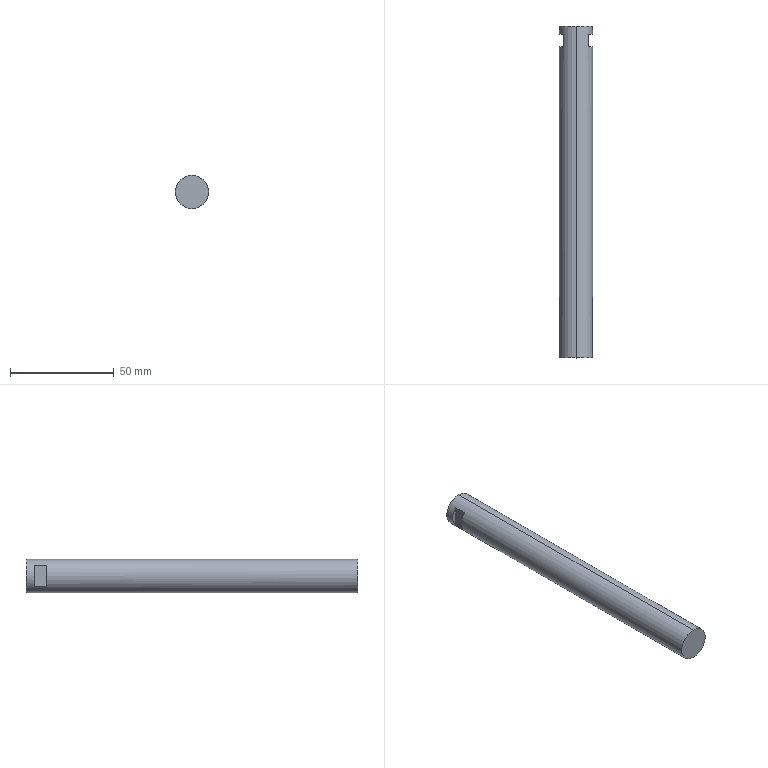Part | STEP file | 1 solid | 10 faces | box 16 x 160 x 16 mm | volume 31996 mm3 | plane 8 | cylinder 2 | commonest cylinder face diameters 16 x2
STEP:
#1=CARTESIAN_POINT('',(0.,0.,0.));
#2=DIRECTION('',(0.,0.,1.));
#3=DIRECTION('',(1.,0.,0.));
#4=AXIS2_PLACEMENT_3D('',#1,#2,#3);
#5=CARTESIAN_POINT('',(6.,156.,5.292));
#6=VERTEX_POINT('',#5);
#7=CARTESIAN_POINT('',(6.,156.,-5.292));
#8=VERTEX_POINT('',#7);
#9=CARTESIAN_POINT('',(0.,156.,0.));
#10=DIRECTION('',(0.,1.,0.));
#11=DIRECTION('',(0.,0.,1.));
#12=AXIS2_PLACEMENT_3D('',#9,#10,#11);
#13=CIRCLE('',#12,8.);
#14=CARTESIAN_POINT('',(0.,160.,0.));
#15=DIRECTION('',(0.,-1.,0.));
#16=DIRECTION('',(0.,0.,-1.));
#17=AXIS2_PLACEMENT_3D('',#14,#15,#16);
#18=CYLINDRICAL_SURFACE('',#17,8.);
#19=CARTESIAN_POINT('',(3.142,4.));
#20=DIRECTION('',(-1.,0.));
#21=VECTOR('',#20,1.);
#22=LINE('',#19,#21);
#23=(GEOMETRIC_REPRESENTATION_CONTEXT(2)PARAMETRIC_REPRESENTATION_CONTEXT()REPRESENTATION_CONTEXT('',''));
#24=DEFINITIONAL_REPRESENTATION('',(#22),#23);
#25=PCURVE('',#18,#24);
#26=CARTESIAN_POINT('',(14.,156.,-12.));
#27=DIRECTION('',(0.,1.,0.));
#28=DIRECTION('',(0.,0.,1.));
#29=AXIS2_PLACEMENT_3D('',#26,#27,#28);
#30=PLANE('',#29);
#31=CARTESIAN_POINT('',(12.,-14.));
#32=DIRECTION('',(1.,0.));
#33=AXIS2_PLACEMENT_2D('',#31,#32);
#34=CIRCLE('',#33,8.);
#35=(GEOMETRIC_REPRESENTATION_CONTEXT(2)PARAMETRIC_REPRESENTATION_CONTEXT()REPRESENTATION_CONTEXT('',''));
#36=DEFINITIONAL_REPRESENTATION('',(#34),#35);
#37=PCURVE('',#30,#36);
#38=SURFACE_CURVE('',#13,(#25,#37),.PCURVE_S1.);
#39=EDGE_CURVE('',#6,#8,#38,.T.);
#40=ORIENTED_EDGE('',*,*,#39,.T.);
#41=CARTESIAN_POINT('',(6.,150.,-5.292));
#42=VERTEX_POINT('',#41);
#43=CARTESIAN_POINT('',(6.,160.,-5.292));
#44=DIRECTION('',(0.,-1.,0.));
#45=VECTOR('',#44,1.);
#46=LINE('',#43,#45);
#47=CARTESIAN_POINT('',(0.8481,0.));
#48=DIRECTION('',(0.,1.));
#49=VECTOR('',#48,1.);
#50=LINE('',#47,#49);
#51=(GEOMETRIC_REPRESENTATION_CONTEXT(2)PARAMETRIC_REPRESENTATION_CONTEXT()REPRESENTATION_CONTEXT('',''));
#52=DEFINITIONAL_REPRESENTATION('',(#50),#51);
#53=PCURVE('',#18,#52);
#54=CARTESIAN_POINT('',(6.,156.,-12.));
#55=DIRECTION('',(-1.,0.,0.));
#56=DIRECTION('',(0.,-1.,0.));
#57=AXIS2_PLACEMENT_3D('',#54,#55,#56);
#58=PLANE('',#57);
#59=CARTESIAN_POINT('',(-4.,6.708));
#60=DIRECTION('',(1.,0.));
#61=VECTOR('',#60,1.);
#62=LINE('',#59,#61);
#63=(GEOMETRIC_REPRESENTATION_CONTEXT(2)PARAMETRIC_REPRESENTATION_CONTEXT()REPRESENTATION_CONTEXT('',''));
#64=DEFINITIONAL_REPRESENTATION('',(#62),#63);
#65=PCURVE('',#58,#64);
#66=SURFACE_CURVE('',#46,(#53,#65),.PCURVE_S1.);
#67=EDGE_CURVE('',#8,#42,#66,.T.);
#68=ORIENTED_EDGE('',*,*,#67,.T.);
#69=CARTESIAN_POINT('',(6.,150.,5.292));
#70=VERTEX_POINT('',#69);
#71=CARTESIAN_POINT('',(0.,150.,0.));
#72=DIRECTION('',(0.,-1.,0.));
#73=DIRECTION('',(0.,0.,-1.));
#74=AXIS2_PLACEMENT_3D('',#71,#72,#73);
#75=CIRCLE('',#74,8.);
#76=CARTESIAN_POINT('',(0.,10.));
#77=DIRECTION('',(1.,0.));
#78=VECTOR('',#77,1.);
#79=LINE('',#76,#78);
#80=(GEOMETRIC_REPRESENTATION_CONTEXT(2)PARAMETRIC_REPRESENTATION_CONTEXT()REPRESENTATION_CONTEXT('',''));
#81=DEFINITIONAL_REPRESENTATION('',(#79),#80);
#82=PCURVE('',#18,#81);
#83=CARTESIAN_POINT('',(14.,150.,-12.));
#84=DIRECTION('',(0.,-1.,0.));
#85=DIRECTION('',(0.,0.,-1.));
#86=AXIS2_PLACEMENT_3D('',#83,#84,#85);
#87=PLANE('',#86);
#88=CARTESIAN_POINT('',(-12.,-14.));
#89=DIRECTION('',(1.,0.));
#90=AXIS2_PLACEMENT_2D('',#88,#89);
#91=CIRCLE('',#90,8.);
#92=(GEOMETRIC_REPRESENTATION_CONTEXT(2)PARAMETRIC_REPRESENTATION_CONTEXT()REPRESENTATION_CONTEXT('',''));
#93=DEFINITIONAL_REPRESENTATION('',(#91),#92);
#94=PCURVE('',#87,#93);
#95=SURFACE_CURVE('',#75,(#82,#94),.PCURVE_S1.);
#96=EDGE_CURVE('',#42,#70,#95,.T.);
#97=ORIENTED_EDGE('',*,*,#96,.T.);
#98=CARTESIAN_POINT('',(6.,160.,5.292));
#99=DIRECTION('',(0.,1.,0.));
#100=VECTOR('',#99,1.);
#101=LINE('',#98,#100);
#102=CARTESIAN_POINT('',(2.294,0.));
#103=DIRECTION('',(0.,-1.));
#104=VECTOR('',#103,1.);
#105=LINE('',#102,#104);
#106=(GEOMETRIC_REPRESENTATION_CONTEXT(2)PARAMETRIC_REPRESENTATION_CONTEXT()REPRESENTATION_CONTEXT('',''));
#107=DEFINITIONAL_REPRESENTATION('',(#105),#106);
#108=PCURVE('',#18,#107);
#109=CARTESIAN_POINT('',(-4.,17.292));
#110=DIRECTION('',(-1.,0.));
#111=VECTOR('',#110,1.);
#112=LINE('',#109,#111);
#113=(GEOMETRIC_REPRESENTATION_CONTEXT(2)PARAMETRIC_REPRESENTATION_CONTEXT()REPRESENTATION_CONTEXT('',''));
#114=DEFINITIONAL_REPRESENTATION('',(#112),#113);
#115=PCURVE('',#58,#114);
#116=SURFACE_CURVE('',#101,(#108,#115),.PCURVE_S1.);
#117=EDGE_CURVE('',#70,#6,#116,.T.);
#118=ORIENTED_EDGE('',*,*,#117,.T.);
#119=EDGE_LOOP('',(#40,#68,#97,#118));
#120=FACE_BOUND('',#119,.T.);
#121=CARTESIAN_POINT('',(0.,160.,8.));
#122=VERTEX_POINT('',#121);
#123=CARTESIAN_POINT('',(0.,160.,-8.));
#124=VERTEX_POINT('',#123);
#125=CARTESIAN_POINT('',(0.,160.,0.));
#126=DIRECTION('',(0.,1.,0.));
#127=DIRECTION('',(0.,0.,1.));
#128=AXIS2_PLACEMENT_3D('',#125,#126,#127);
#129=CIRCLE('',#128,8.);
#130=CARTESIAN_POINT('',(3.142,0.));
#131=DIRECTION('',(-1.,0.));
#132=VECTOR('',#131,1.);
#133=LINE('',#130,#132);
#134=(GEOMETRIC_REPRESENTATION_CONTEXT(2)PARAMETRIC_REPRESENTATION_CONTEXT()REPRESENTATION_CONTEXT('',''));
#135=DEFINITIONAL_REPRESENTATION('',(#133),#134);
#136=PCURVE('',#18,#135);
#137=CARTESIAN_POINT('',(0.,160.,0.));
#138=DIRECTION('',(0.,1.,0.));
#139=DIRECTION('',(0.,0.,1.));
#140=AXIS2_PLACEMENT_3D('',#137,#138,#139);
#141=PLANE('',#140);
#142=CARTESIAN_POINT('',(0.,0.));
#143=DIRECTION('',(1.,0.));
#144=AXIS2_PLACEMENT_2D('',#142,#143);
#145=CIRCLE('',#144,8.);
#146=(GEOMETRIC_REPRESENTATION_CONTEXT(2)PARAMETRIC_REPRESENTATION_CONTEXT()REPRESENTATION_CONTEXT('',''));
#147=DEFINITIONAL_REPRESENTATION('',(#145),#146);
#148=PCURVE('',#141,#147);
#149=SURFACE_CURVE('',#129,(#136,#148),.PCURVE_S1.);
#150=EDGE_CURVE('',#122,#124,#149,.T.);
#151=ORIENTED_EDGE('',*,*,#150,.F.);
#152=CARTESIAN_POINT('',(0.,0.,8.));
#153=VERTEX_POINT('',#152);
#154=CARTESIAN_POINT('',(0.,160.,8.));
#155=DIRECTION('',(0.,-1.,0.));
#156=VECTOR('',#155,1.);
#157=LINE('',#154,#156);
#158=CARTESIAN_POINT('',(3.142,0.));
#159=DIRECTION('',(0.,1.));
#160=VECTOR('',#159,1.);
#161=LINE('',#158,#160);
#162=(GEOMETRIC_REPRESENTATION_CONTEXT(2)PARAMETRIC_REPRESENTATION_CONTEXT()REPRESENTATION_CONTEXT('',''));
#163=DEFINITIONAL_REPRESENTATION('',(#161),#162);
#164=PCURVE('',#18,#163);
#165=CARTESIAN_POINT('',(0.,160.,0.));
#166=DIRECTION('',(0.,-1.,0.));
#167=DIRECTION('',(0.,0.,-1.));
#168=AXIS2_PLACEMENT_3D('',#165,#166,#167);
#169=CYLINDRICAL_SURFACE('',#168,8.);
#170=CARTESIAN_POINT('',(3.142,0.));
#171=DIRECTION('',(0.,1.));
#172=VECTOR('',#171,1.);
#173=LINE('',#170,#172);
#174=(GEOMETRIC_REPRESENTATION_CONTEXT(2)PARAMETRIC_REPRESENTATION_CONTEXT()REPRESENTATION_CONTEXT('',''));
#175=DEFINITIONAL_REPRESENTATION('',(#173),#174);
#176=PCURVE('',#169,#175);
#177=SURFACE_CURVE('',#157,(#164,#176),.PCURVE_S1.);
#178=EDGE_CURVE('',#122,#153,#177,.T.);
#179=ORIENTED_EDGE('',*,*,#178,.T.);
#180=CARTESIAN_POINT('',(0.,0.,-8.));
#181=VERTEX_POINT('',#180);
#182=CARTESIAN_POINT('',(0.,0.,0.));
#183=DIRECTION('',(0.,1.,0.));
#184=DIRECTION('',(0.,0.,1.));
#185=AXIS2_PLACEMENT_3D('',#182,#183,#184);
#186=CIRCLE('',#185,8.);
#187=CARTESIAN_POINT('',(3.142,160.));
#188=DIRECTION('',(-1.,0.));
#189=VECTOR('',#188,1.);
#190=LINE('',#187,#189);
#191=(GEOMETRIC_REPRESENTATION_CONTEXT(2)PARAMETRIC_REPRESENTATION_CONTEXT()REPRESENTATION_CONTEXT('',''));
#192=DEFINITIONAL_REPRESENTATION('',(#190),#191);
#193=PCURVE('',#18,#192);
#194=CARTESIAN_POINT('',(0.,0.,0.));
#195=DIRECTION('',(0.,1.,0.));
#196=DIRECTION('',(0.,0.,1.));
#197=AXIS2_PLACEMENT_3D('',#194,#195,#196);
#198=PLANE('',#197);
#199=CARTESIAN_POINT('',(0.,0.));
#200=DIRECTION('',(1.,0.));
#201=AXIS2_PLACEMENT_2D('',#199,#200);
#202=CIRCLE('',#201,8.);
#203=(GEOMETRIC_REPRESENTATION_CONTEXT(2)PARAMETRIC_REPRESENTATION_CONTEXT()REPRESENTATION_CONTEXT('',''));
#204=DEFINITIONAL_REPRESENTATION('',(#202),#203);
#205=PCURVE('',#198,#204);
#206=SURFACE_CURVE('',#186,(#193,#205),.PCURVE_S1.);
#207=EDGE_CURVE('',#153,#181,#206,.T.);
#208=ORIENTED_EDGE('',*,*,#207,.T.);
#209=CARTESIAN_POINT('',(0.,160.,-8.));
#210=DIRECTION('',(0.,-1.,0.));
#211=VECTOR('',#210,1.);
#212=LINE('',#209,#211);
#213=CARTESIAN_POINT('',(0.,0.));
#214=DIRECTION('',(0.,1.));
#215=VECTOR('',#214,1.);
#216=LINE('',#213,#215);
#217=(GEOMETRIC_REPRESENTATION_CONTEXT(2)PARAMETRIC_REPRESENTATION_CONTEXT()REPRESENTATION_CONTEXT('',''));
#218=DEFINITIONAL_REPRESENTATION('',(#216),#217);
#219=PCURVE('',#18,#218);
#220=CARTESIAN_POINT('',(6.283,0.));
#221=DIRECTION('',(0.,1.));
#222=VECTOR('',#221,1.);
#223=LINE('',#220,#222);
#224=(GEOMETRIC_REPRESENTATION_CONTEXT(2)PARAMETRIC_REPRESENTATION_CONTEXT()REPRESENTATION_CONTEXT('',''));
#225=DEFINITIONAL_REPRESENTATION('',(#223),#224);
#226=PCURVE('',#169,#225);
#227=SURFACE_CURVE('',#212,(#219,#226),.PCURVE_S1.);
#228=EDGE_CURVE('',#124,#181,#227,.T.);
#229=ORIENTED_EDGE('',*,*,#228,.F.);
#230=EDGE_LOOP('',(#151,#179,#208,#229));
#231=FACE_BOUND('',#230,.T.);
#232=ADVANCED_FACE('',(#120,#231),#18,.T.);
#233=ORIENTED_EDGE('',*,*,#178,.F.);
#234=CARTESIAN_POINT('',(0.,160.,0.));
#235=DIRECTION('',(0.,1.,0.));
#236=DIRECTION('',(0.,0.,1.));
#237=AXIS2_PLACEMENT_3D('',#234,#235,#236);
#238=CIRCLE('',#237,8.);
#239=CARTESIAN_POINT('',(9.425,0.));
#240=DIRECTION('',(-1.,0.));
#241=VECTOR('',#240,1.);
#242=LINE('',#239,#241);
#243=(GEOMETRIC_REPRESENTATION_CONTEXT(2)PARAMETRIC_REPRESENTATION_CONTEXT()REPRESENTATION_CONTEXT('',''));
#244=DEFINITIONAL_REPRESENTATION('',(#242),#243);
#245=PCURVE('',#169,#244);
#246=CARTESIAN_POINT('',(0.,0.));
#247=DIRECTION('',(1.,0.));
#248=AXIS2_PLACEMENT_2D('',#246,#247);
#249=CIRCLE('',#248,8.);
#250=(GEOMETRIC_REPRESENTATION_CONTEXT(2)PARAMETRIC_REPRESENTATION_CONTEXT()REPRESENTATION_CONTEXT('',''));
#251=DEFINITIONAL_REPRESENTATION('',(#249),#250);
#252=PCURVE('',#141,#251);
#253=SURFACE_CURVE('',#238,(#245,#252),.PCURVE_S1.);
#254=EDGE_CURVE('',#124,#122,#253,.T.);
#255=ORIENTED_EDGE('',*,*,#254,.F.);
#256=ORIENTED_EDGE('',*,*,#228,.T.);
#257=CARTESIAN_POINT('',(0.,0.,0.));
#258=DIRECTION('',(0.,1.,0.));
#259=DIRECTION('',(0.,0.,1.));
#260=AXIS2_PLACEMENT_3D('',#257,#258,#259);
#261=CIRCLE('',#260,8.);
#262=CARTESIAN_POINT('',(9.425,160.));
#263=DIRECTION('',(-1.,0.));
#264=VECTOR('',#263,1.);
#265=LINE('',#262,#264);
#266=(GEOMETRIC_REPRESENTATION_CONTEXT(2)PARAMETRIC_REPRESENTATION_CONTEXT()REPRESENTATION_CONTEXT('',''));
#267=DEFINITIONAL_REPRESENTATION('',(#265),#266);
#268=PCURVE('',#169,#267);
#269=CARTESIAN_POINT('',(0.,0.));
#270=DIRECTION('',(1.,0.));
#271=AXIS2_PLACEMENT_2D('',#269,#270);
#272=CIRCLE('',#271,8.);
#273=(GEOMETRIC_REPRESENTATION_CONTEXT(2)PARAMETRIC_REPRESENTATION_CONTEXT()REPRESENTATION_CONTEXT('',''));
#274=DEFINITIONAL_REPRESENTATION('',(#272),#273);
#275=PCURVE('',#198,#274);
#276=SURFACE_CURVE('',#261,(#268,#275),.PCURVE_S1.);
#277=EDGE_CURVE('',#181,#153,#276,.T.);
#278=ORIENTED_EDGE('',*,*,#277,.T.);
#279=EDGE_LOOP('',(#233,#255,#256,#278));
#280=FACE_BOUND('',#279,.T.);
#281=CARTESIAN_POINT('',(-6.,150.,-5.292));
#282=VERTEX_POINT('',#281);
#283=CARTESIAN_POINT('',(-6.,156.,-5.292));
#284=VERTEX_POINT('',#283);
#285=CARTESIAN_POINT('',(-6.,160.,-5.292));
#286=DIRECTION('',(0.,1.,0.));
#287=VECTOR('',#286,1.);
#288=LINE('',#285,#287);
#289=CARTESIAN_POINT('',(5.435,0.));
#290=DIRECTION('',(0.,-1.));
#291=VECTOR('',#290,1.);
#292=LINE('',#289,#291);
#293=(GEOMETRIC_REPRESENTATION_CONTEXT(2)PARAMETRIC_REPRESENTATION_CONTEXT()REPRESENTATION_CONTEXT('',''));
#294=DEFINITIONAL_REPRESENTATION('',(#292),#293);
#295=PCURVE('',#169,#294);
#296=CARTESIAN_POINT('',(-6.,156.,-12.));
#297=DIRECTION('',(1.,0.,0.));
#298=DIRECTION('',(0.,1.,0.));
#299=AXIS2_PLACEMENT_3D('',#296,#297,#298);
#300=PLANE('',#299);
#301=CARTESIAN_POINT('',(4.,6.708));
#302=DIRECTION('',(1.,0.));
#303=VECTOR('',#302,1.);
#304=LINE('',#301,#303);
#305=(GEOMETRIC_REPRESENTATION_CONTEXT(2)PARAMETRIC_REPRESENTATION_CONTEXT()REPRESENTATION_CONTEXT('',''));
#306=DEFINITIONAL_REPRESENTATION('',(#304),#305);
#307=PCURVE('',#300,#306);
#308=SURFACE_CURVE('',#288,(#295,#307),.PCURVE_S1.);
#309=EDGE_CURVE('',#282,#284,#308,.T.);
#310=ORIENTED_EDGE('',*,*,#309,.T.);
#311=CARTESIAN_POINT('',(-6.,156.,5.292));
#312=VERTEX_POINT('',#311);
#313=CARTESIAN_POINT('',(0.,156.,0.));
#314=DIRECTION('',(0.,1.,0.));
#315=DIRECTION('',(0.,0.,1.));
#316=AXIS2_PLACEMENT_3D('',#313,#314,#315);
#317=CIRCLE('',#316,8.);
#318=CARTESIAN_POINT('',(9.425,4.));
#319=DIRECTION('',(-1.,0.));
#320=VECTOR('',#319,1.);
#321=LINE('',#318,#320);
#322=(GEOMETRIC_REPRESENTATION_CONTEXT(2)PARAMETRIC_REPRESENTATION_CONTEXT()REPRESENTATION_CONTEXT('',''));
#323=DEFINITIONAL_REPRESENTATION('',(#321),#322);
#324=PCURVE('',#169,#323);
#325=CARTESIAN_POINT('',(-14.,156.,-12.));
#326=DIRECTION('',(0.,1.,0.));
#327=DIRECTION('',(0.,0.,1.));
#328=AXIS2_PLACEMENT_3D('',#325,#326,#327);
#329=PLANE('',#328);
#330=CARTESIAN_POINT('',(12.,14.));
#331=DIRECTION('',(1.,0.));
#332=AXIS2_PLACEMENT_2D('',#330,#331);
#333=CIRCLE('',#332,8.);
#334=(GEOMETRIC_REPRESENTATION_CONTEXT(2)PARAMETRIC_REPRESENTATION_CONTEXT()REPRESENTATION_CONTEXT('',''));
#335=DEFINITIONAL_REPRESENTATION('',(#333),#334);
#336=PCURVE('',#329,#335);
#337=SURFACE_CURVE('',#317,(#324,#336),.PCURVE_S1.);
#338=EDGE_CURVE('',#284,#312,#337,.T.);
#339=ORIENTED_EDGE('',*,*,#338,.T.);
#340=CARTESIAN_POINT('',(-6.,150.,5.292));
#341=VERTEX_POINT('',#340);
#342=CARTESIAN_POINT('',(-6.,160.,5.292));
#343=DIRECTION('',(0.,-1.,0.));
#344=VECTOR('',#343,1.);
#345=LINE('',#342,#344);
#346=CARTESIAN_POINT('',(3.99,0.));
#347=DIRECTION('',(0.,1.));
#348=VECTOR('',#347,1.);
#349=LINE('',#346,#348);
#350=(GEOMETRIC_REPRESENTATION_CONTEXT(2)PARAMETRIC_REPRESENTATION_CONTEXT()REPRESENTATION_CONTEXT('',''));
#351=DEFINITIONAL_REPRESENTATION('',(#349),#350);
#352=PCURVE('',#169,#351);
#353=CARTESIAN_POINT('',(4.,17.292));
#354=DIRECTION('',(-1.,0.));
#355=VECTOR('',#354,1.);
#356=LINE('',#353,#355);
#357=(GEOMETRIC_REPRESENTATION_CONTEXT(2)PARAMETRIC_REPRESENTATION_CONTEXT()REPRESENTATION_CONTEXT('',''));
#358=DEFINITIONAL_REPRESENTATION('',(#356),#357);
#359=PCURVE('',#300,#358);
#360=SURFACE_CURVE('',#345,(#352,#359),.PCURVE_S1.);
#361=EDGE_CURVE('',#312,#341,#360,.T.);
#362=ORIENTED_EDGE('',*,*,#361,.T.);
#363=CARTESIAN_POINT('',(0.,150.,0.));
#364=DIRECTION('',(0.,-1.,0.));
#365=DIRECTION('',(0.,0.,-1.));
#366=AXIS2_PLACEMENT_3D('',#363,#364,#365);
#367=CIRCLE('',#366,8.);
#368=CARTESIAN_POINT('',(0.,10.));
#369=DIRECTION('',(1.,0.));
#370=VECTOR('',#369,1.);
#371=LINE('',#368,#370);
#372=(GEOMETRIC_REPRESENTATION_CONTEXT(2)PARAMETRIC_REPRESENTATION_CONTEXT()REPRESENTATION_CONTEXT('',''));
#373=DEFINITIONAL_REPRESENTATION('',(#371),#372);
#374=PCURVE('',#169,#373);
#375=CARTESIAN_POINT('',(-14.,150.,-12.));
#376=DIRECTION('',(0.,-1.,0.));
#377=DIRECTION('',(0.,0.,-1.));
#378=AXIS2_PLACEMENT_3D('',#375,#376,#377);
#379=PLANE('',#378);
#380=CARTESIAN_POINT('',(-12.,14.));
#381=DIRECTION('',(1.,0.));
#382=AXIS2_PLACEMENT_2D('',#380,#381);
#383=CIRCLE('',#382,8.);
#384=(GEOMETRIC_REPRESENTATION_CONTEXT(2)PARAMETRIC_REPRESENTATION_CONTEXT()REPRESENTATION_CONTEXT('',''));
#385=DEFINITIONAL_REPRESENTATION('',(#383),#384);
#386=PCURVE('',#379,#385);
#387=SURFACE_CURVE('',#367,(#374,#386),.PCURVE_S1.);
#388=EDGE_CURVE('',#341,#282,#387,.T.);
#389=ORIENTED_EDGE('',*,*,#388,.T.);
#390=EDGE_LOOP('',(#310,#339,#362,#389));
#391=FACE_BOUND('',#390,.T.);
#392=ADVANCED_FACE('',(#280,#391),#169,.T.);
#393=ORIENTED_EDGE('',*,*,#254,.T.);
#394=ORIENTED_EDGE('',*,*,#150,.T.);
#395=EDGE_LOOP('',(#393,#394));
#396=FACE_BOUND('',#395,.T.);
#397=ADVANCED_FACE('',(#396),#141,.T.);
#398=ORIENTED_EDGE('',*,*,#277,.F.);
#399=ORIENTED_EDGE('',*,*,#207,.F.);
#400=EDGE_LOOP('',(#398,#399));
#401=FACE_BOUND('',#400,.T.);
#402=ADVANCED_FACE('',(#401),#198,.F.);
#403=CARTESIAN_POINT('',(-6.,156.,-12.));
#404=DIRECTION('',(0.,0.,1.));
#405=VECTOR('',#404,1.);
#406=LINE('',#403,#405);
#407=CARTESIAN_POINT('',(0.,8.));
#408=DIRECTION('',(1.,0.));
#409=VECTOR('',#408,1.);
#410=LINE('',#407,#409);
#411=(GEOMETRIC_REPRESENTATION_CONTEXT(2)PARAMETRIC_REPRESENTATION_CONTEXT()REPRESENTATION_CONTEXT('',''));
#412=DEFINITIONAL_REPRESENTATION('',(#410),#411);
#413=PCURVE('',#329,#412);
#414=CARTESIAN_POINT('',(0.,0.));
#415=DIRECTION('',(0.,1.));
#416=VECTOR('',#415,1.);
#417=LINE('',#414,#416);
#418=(GEOMETRIC_REPRESENTATION_CONTEXT(2)PARAMETRIC_REPRESENTATION_CONTEXT()REPRESENTATION_CONTEXT('',''));
#419=DEFINITIONAL_REPRESENTATION('',(#417),#418);
#420=PCURVE('',#300,#419);
#421=SURFACE_CURVE('',#406,(#413,#420),.PCURVE_S1.);
#422=EDGE_CURVE('',#284,#312,#421,.T.);
#423=ORIENTED_EDGE('',*,*,#422,.T.);
#424=ORIENTED_EDGE('',*,*,#338,.F.);
#425=EDGE_LOOP('',(#423,#424));
#426=FACE_BOUND('',#425,.T.);
#427=ADVANCED_FACE('',(#426),#329,.F.);
#428=ORIENTED_EDGE('',*,*,#422,.F.);
#429=ORIENTED_EDGE('',*,*,#309,.F.);
#430=CARTESIAN_POINT('',(-6.,150.,-12.));
#431=DIRECTION('',(0.,0.,1.));
#432=VECTOR('',#431,1.);
#433=LINE('',#430,#432);
#434=CARTESIAN_POINT('',(-6.,0.));
#435=DIRECTION('',(0.,1.));
#436=VECTOR('',#435,1.);
#437=LINE('',#434,#436);
#438=(GEOMETRIC_REPRESENTATION_CONTEXT(2)PARAMETRIC_REPRESENTATION_CONTEXT()REPRESENTATION_CONTEXT('',''));
#439=DEFINITIONAL_REPRESENTATION('',(#437),#438);
#440=PCURVE('',#300,#439);
#441=CARTESIAN_POINT('',(0.,8.));
#442=DIRECTION('',(-1.,0.));
#443=VECTOR('',#442,1.);
#444=LINE('',#441,#443);
#445=(GEOMETRIC_REPRESENTATION_CONTEXT(2)PARAMETRIC_REPRESENTATION_CONTEXT()REPRESENTATION_CONTEXT('',''));
#446=DEFINITIONAL_REPRESENTATION('',(#444),#445);
#447=PCURVE('',#379,#446);
#448=SURFACE_CURVE('',#433,(#440,#447),.PCURVE_S1.);
#449=EDGE_CURVE('',#282,#341,#448,.T.);
#450=ORIENTED_EDGE('',*,*,#449,.T.);
#451=ORIENTED_EDGE('',*,*,#361,.F.);
#452=EDGE_LOOP('',(#428,#429,#450,#451));
#453=FACE_BOUND('',#452,.T.);
#454=ADVANCED_FACE('',(#453),#300,.F.);
#455=ORIENTED_EDGE('',*,*,#449,.F.);
#456=ORIENTED_EDGE('',*,*,#388,.F.);
#457=EDGE_LOOP('',(#455,#456));
#458=FACE_BOUND('',#457,.T.);
#459=ADVANCED_FACE('',(#458),#379,.F.);
#460=CARTESIAN_POINT('',(6.,156.,-12.));
#461=DIRECTION('',(0.,0.,1.));
#462=VECTOR('',#461,1.);
#463=LINE('',#460,#462);
#464=CARTESIAN_POINT('',(0.,-8.));
#465=DIRECTION('',(1.,0.));
#466=VECTOR('',#465,1.);
#467=LINE('',#464,#466);
#468=(GEOMETRIC_REPRESENTATION_CONTEXT(2)PARAMETRIC_REPRESENTATION_CONTEXT()REPRESENTATION_CONTEXT('',''));
#469=DEFINITIONAL_REPRESENTATION('',(#467),#468);
#470=PCURVE('',#30,#469);
#471=CARTESIAN_POINT('',(0.,0.));
#472=DIRECTION('',(0.,1.));
#473=VECTOR('',#472,1.);
#474=LINE('',#471,#473);
#475=(GEOMETRIC_REPRESENTATION_CONTEXT(2)PARAMETRIC_REPRESENTATION_CONTEXT()REPRESENTATION_CONTEXT('',''));
#476=DEFINITIONAL_REPRESENTATION('',(#474),#475);
#477=PCURVE('',#58,#476);
#478=SURFACE_CURVE('',#463,(#470,#477),.PCURVE_S1.);
#479=EDGE_CURVE('',#8,#6,#478,.T.);
#480=ORIENTED_EDGE('',*,*,#479,.F.);
#481=ORIENTED_EDGE('',*,*,#39,.F.);
#482=EDGE_LOOP('',(#480,#481));
#483=FACE_BOUND('',#482,.T.);
#484=ADVANCED_FACE('',(#483),#30,.F.);
#485=CARTESIAN_POINT('',(6.,150.,-12.));
#486=DIRECTION('',(0.,0.,1.));
#487=VECTOR('',#486,1.);
#488=LINE('',#485,#487);
#489=CARTESIAN_POINT('',(0.,-8.));
#490=DIRECTION('',(-1.,0.));
#491=VECTOR('',#490,1.);
#492=LINE('',#489,#491);
#493=(GEOMETRIC_REPRESENTATION_CONTEXT(2)PARAMETRIC_REPRESENTATION_CONTEXT()REPRESENTATION_CONTEXT('',''));
#494=DEFINITIONAL_REPRESENTATION('',(#492),#493);
#495=PCURVE('',#87,#494);
#496=CARTESIAN_POINT('',(6.,0.));
#497=DIRECTION('',(0.,1.));
#498=VECTOR('',#497,1.);
#499=LINE('',#496,#498);
#500=(GEOMETRIC_REPRESENTATION_CONTEXT(2)PARAMETRIC_REPRESENTATION_CONTEXT()REPRESENTATION_CONTEXT('',''));
#501=DEFINITIONAL_REPRESENTATION('',(#499),#500);
#502=PCURVE('',#58,#501);
#503=SURFACE_CURVE('',#488,(#495,#502),.PCURVE_S1.);
#504=EDGE_CURVE('',#42,#70,#503,.T.);
#505=ORIENTED_EDGE('',*,*,#504,.T.);
#506=ORIENTED_EDGE('',*,*,#96,.F.);
#507=EDGE_LOOP('',(#505,#506));
#508=FACE_BOUND('',#507,.T.);
#509=ADVANCED_FACE('',(#508),#87,.F.);
#510=ORIENTED_EDGE('',*,*,#479,.T.);
#511=ORIENTED_EDGE('',*,*,#117,.F.);
#512=ORIENTED_EDGE('',*,*,#504,.F.);
#513=ORIENTED_EDGE('',*,*,#67,.F.);
#514=EDGE_LOOP('',(#510,#511,#512,#513));
#515=FACE_BOUND('',#514,.T.);
#516=ADVANCED_FACE('',(#515),#58,.F.);
#517=CLOSED_SHELL('',(#232,#392,#397,#402,#427,#454,#459,#484,#509,#516));
#518=MANIFOLD_SOLID_BREP('',#517);
#519=(LENGTH_UNIT()NAMED_UNIT(*)SI_UNIT(.MILLI.,.METRE.));
#520=UNCERTAINTY_MEASURE_WITH_UNIT(LENGTH_MEASURE(0.0000001),#519,'','');
#521=(NAMED_UNIT(*)PLANE_ANGLE_UNIT()SI_UNIT($,.RADIAN.));
#522=(NAMED_UNIT(*)SI_UNIT($,.STERADIAN.)SOLID_ANGLE_UNIT());
#523=(GEOMETRIC_REPRESENTATION_CONTEXT(3)GLOBAL_UNCERTAINTY_ASSIGNED_CONTEXT((#520))GLOBAL_UNIT_ASSIGNED_CONTEXT((#519,#521,#522))REPRESENTATION_CONTEXT('',''));
#524=ADVANCED_BREP_SHAPE_REPRESENTATION('',(#4,#518),#523);